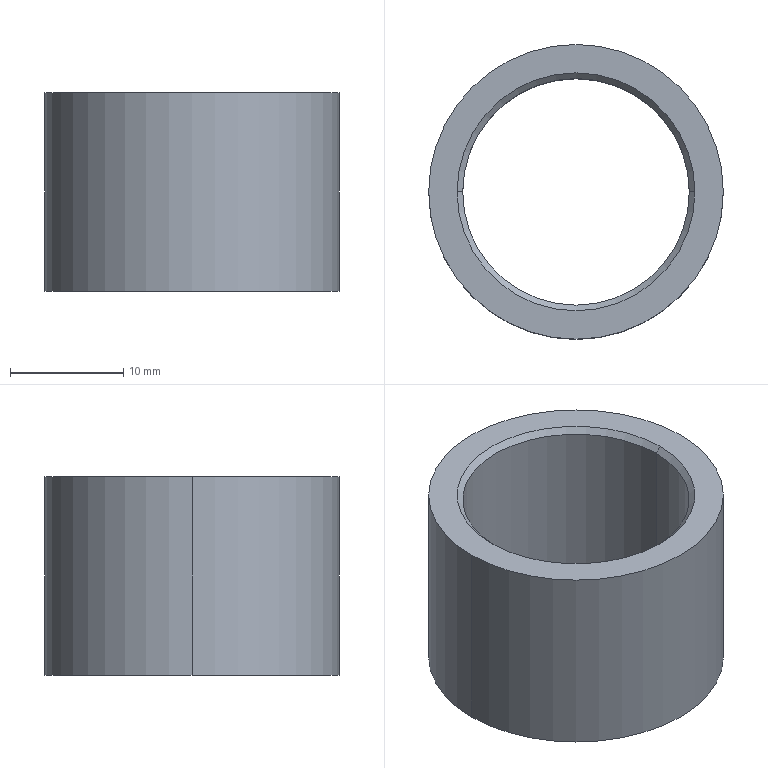Part | SolidWorks | features Chamfer 1, Extrusion 1 | 1 solid | 10 faces | box 26 x 26 x 17.5 mm | volume 3778 mm3 | cone 4 | cylinder 4 | plane 2 | commonest cylinder face diameters 20 x2 26 x2
STEP:
#1=CARTESIAN_POINT('',(-10.,0.,17.));
#2=VERTEX_POINT('',#1);
#3=CARTESIAN_POINT('',(10.,0.,17.));
#4=VERTEX_POINT('',#3);
#5=CARTESIAN_POINT('',(0.,0.,17.));
#6=DIRECTION('',(0.,0.,1.));
#7=DIRECTION('',(1.,0.,0.));
#8=AXIS2_PLACEMENT_3D('',#5,#6,#7);
#9=CIRCLE('',#8,10.);
#10=EDGE_CURVE('',#2,#4,#9,.T.);
#11=ORIENTED_EDGE('',*,*,#10,.F.);
#12=CARTESIAN_POINT('',(-10.5,0.,17.5));
#13=VERTEX_POINT('',#12);
#14=CARTESIAN_POINT('',(-10.,0.,17.));
#15=DIRECTION('',(-0.7071,0.,0.7071));
#16=VECTOR('',#15,1000.);
#17=LINE('',#14,#16);
#18=EDGE_CURVE('',#2,#13,#17,.T.);
#19=ORIENTED_EDGE('',*,*,#18,.T.);
#20=CARTESIAN_POINT('',(10.5,0.,17.5));
#21=VERTEX_POINT('',#20);
#22=CARTESIAN_POINT('',(0.,0.,17.5));
#23=DIRECTION('',(0.,0.,-1.));
#24=DIRECTION('',(1.,0.,0.));
#25=AXIS2_PLACEMENT_3D('',#22,#23,#24);
#26=CIRCLE('',#25,10.5);
#27=EDGE_CURVE('',#21,#13,#26,.T.);
#28=ORIENTED_EDGE('',*,*,#27,.F.);
#29=CARTESIAN_POINT('',(10.,0.,17.));
#30=DIRECTION('',(0.7071,0.,0.7071));
#31=VECTOR('',#30,1000.);
#32=LINE('',#29,#31);
#33=EDGE_CURVE('',#4,#21,#32,.T.);
#34=ORIENTED_EDGE('',*,*,#33,.F.);
#35=EDGE_LOOP('',(#11,#19,#28,#34));
#36=FACE_OUTER_BOUND('',#35,.T.);
#37=CARTESIAN_POINT('',(0.,0.,17.));
#38=DIRECTION('',(0.,0.,1.));
#39=DIRECTION('',(1.,0.,0.));
#40=AXIS2_PLACEMENT_3D('',#37,#38,#39);
#41=CONICAL_SURFACE('',#40,10.,0.7854);
#42=ADVANCED_FACE('',(#36),#41,.F.);
#43=CARTESIAN_POINT('',(10.,0.,0.5));
#44=VERTEX_POINT('',#43);
#45=CARTESIAN_POINT('',(-10.,0.,0.5));
#46=VERTEX_POINT('',#45);
#47=CARTESIAN_POINT('',(0.,0.,0.5));
#48=DIRECTION('',(0.,0.,-1.));
#49=DIRECTION('',(1.,0.,0.));
#50=AXIS2_PLACEMENT_3D('',#47,#48,#49);
#51=CIRCLE('',#50,10.);
#52=EDGE_CURVE('',#44,#46,#51,.T.);
#53=ORIENTED_EDGE('',*,*,#52,.F.);
#54=CARTESIAN_POINT('',(10.5,0.,0.));
#55=VERTEX_POINT('',#54);
#56=CARTESIAN_POINT('',(10.5,0.,0.));
#57=DIRECTION('',(0.7071,0.,-0.7071));
#58=VECTOR('',#57,1000.);
#59=LINE('',#56,#58);
#60=EDGE_CURVE('',#44,#55,#59,.T.);
#61=ORIENTED_EDGE('',*,*,#60,.T.);
#62=CARTESIAN_POINT('',(-10.5,0.,0.));
#63=VERTEX_POINT('',#62);
#64=CARTESIAN_POINT('',(0.,0.,0.));
#65=DIRECTION('',(0.,0.,1.));
#66=DIRECTION('',(1.,0.,0.));
#67=AXIS2_PLACEMENT_3D('',#64,#65,#66);
#68=CIRCLE('',#67,10.5);
#69=EDGE_CURVE('',#63,#55,#68,.T.);
#70=ORIENTED_EDGE('',*,*,#69,.F.);
#71=CARTESIAN_POINT('',(-10.5,0.,0.));
#72=DIRECTION('',(-0.7071,0.,-0.7071));
#73=VECTOR('',#72,1000.);
#74=LINE('',#71,#73);
#75=EDGE_CURVE('',#46,#63,#74,.T.);
#76=ORIENTED_EDGE('',*,*,#75,.F.);
#77=EDGE_LOOP('',(#53,#61,#70,#76));
#78=FACE_OUTER_BOUND('',#77,.T.);
#79=CARTESIAN_POINT('',(0.,0.,0.));
#80=DIRECTION('',(0.,0.,-1.));
#81=DIRECTION('',(-1.,0.,0.));
#82=AXIS2_PLACEMENT_3D('',#79,#80,#81);
#83=CONICAL_SURFACE('',#82,10.5,0.7854);
#84=ADVANCED_FACE('',(#78),#83,.F.);
#85=ORIENTED_EDGE('',*,*,#10,.T.);
#86=CARTESIAN_POINT('',(10.,0.,17.5));
#87=DIRECTION('',(0.,0.,-1.));
#88=VECTOR('',#87,1000.);
#89=LINE('',#86,#88);
#90=EDGE_CURVE('',#4,#44,#89,.T.);
#91=ORIENTED_EDGE('',*,*,#90,.T.);
#92=ORIENTED_EDGE('',*,*,#52,.T.);
#93=CARTESIAN_POINT('',(-10.,0.,17.5));
#94=DIRECTION('',(0.,0.,-1.));
#95=VECTOR('',#94,1000.);
#96=LINE('',#93,#95);
#97=EDGE_CURVE('',#2,#46,#96,.T.);
#98=ORIENTED_EDGE('',*,*,#97,.F.);
#99=EDGE_LOOP('',(#85,#91,#92,#98));
#100=FACE_OUTER_BOUND('',#99,.T.);
#101=CARTESIAN_POINT('',(0.,0.,17.5));
#102=DIRECTION('',(0.,0.,-1.));
#103=DIRECTION('',(-1.,0.,0.));
#104=AXIS2_PLACEMENT_3D('',#101,#102,#103);
#105=CYLINDRICAL_SURFACE('',#104,10.);
#106=ADVANCED_FACE('',(#100),#105,.F.);
#107=CARTESIAN_POINT('',(13.,0.,17.5));
#108=VERTEX_POINT('',#107);
#109=CARTESIAN_POINT('',(-13.,0.,17.5));
#110=VERTEX_POINT('',#109);
#111=CARTESIAN_POINT('',(0.,0.,17.5));
#112=DIRECTION('',(0.,0.,1.));
#113=DIRECTION('',(1.,0.,0.));
#114=AXIS2_PLACEMENT_3D('',#111,#112,#113);
#115=CIRCLE('',#114,13.);
#116=EDGE_CURVE('',#108,#110,#115,.T.);
#117=ORIENTED_EDGE('',*,*,#116,.F.);
#118=CARTESIAN_POINT('',(13.,0.,0.));
#119=VERTEX_POINT('',#118);
#120=CARTESIAN_POINT('',(13.,0.,17.5));
#121=DIRECTION('',(0.,0.,-1.));
#122=VECTOR('',#121,1000.);
#123=LINE('',#120,#122);
#124=EDGE_CURVE('',#108,#119,#123,.T.);
#125=ORIENTED_EDGE('',*,*,#124,.T.);
#126=CARTESIAN_POINT('',(-13.,0.,0.));
#127=VERTEX_POINT('',#126);
#128=CARTESIAN_POINT('',(0.,0.,0.));
#129=DIRECTION('',(0.,0.,1.));
#130=DIRECTION('',(1.,0.,0.));
#131=AXIS2_PLACEMENT_3D('',#128,#129,#130);
#132=CIRCLE('',#131,13.);
#133=EDGE_CURVE('',#119,#127,#132,.T.);
#134=ORIENTED_EDGE('',*,*,#133,.T.);
#135=CARTESIAN_POINT('',(-13.,0.,17.5));
#136=DIRECTION('',(0.,0.,-1.));
#137=VECTOR('',#136,1000.);
#138=LINE('',#135,#137);
#139=EDGE_CURVE('',#110,#127,#138,.T.);
#140=ORIENTED_EDGE('',*,*,#139,.F.);
#141=EDGE_LOOP('',(#117,#125,#134,#140));
#142=FACE_OUTER_BOUND('',#141,.T.);
#143=CARTESIAN_POINT('',(0.,0.,17.5));
#144=DIRECTION('',(0.,0.,-1.));
#145=DIRECTION('',(-1.,0.,0.));
#146=AXIS2_PLACEMENT_3D('',#143,#144,#145);
#147=CYLINDRICAL_SURFACE('',#146,13.);
#148=ADVANCED_FACE('',(#142),#147,.T.);
#149=ORIENTED_EDGE('',*,*,#27,.T.);
#150=CARTESIAN_POINT('',(0.,0.,17.5));
#151=DIRECTION('',(0.,0.,-1.));
#152=DIRECTION('',(1.,0.,0.));
#153=AXIS2_PLACEMENT_3D('',#150,#151,#152);
#154=CIRCLE('',#153,10.5);
#155=EDGE_CURVE('',#13,#21,#154,.T.);
#156=ORIENTED_EDGE('',*,*,#155,.T.);
#157=EDGE_LOOP('',(#149,#156));
#158=FACE_BOUND('',#157,.T.);
#159=CARTESIAN_POINT('',(0.,0.,17.5));
#160=DIRECTION('',(0.,0.,1.));
#161=DIRECTION('',(1.,0.,0.));
#162=AXIS2_PLACEMENT_3D('',#159,#160,#161);
#163=CIRCLE('',#162,13.);
#164=EDGE_CURVE('',#110,#108,#163,.T.);
#165=ORIENTED_EDGE('',*,*,#164,.T.);
#166=ORIENTED_EDGE('',*,*,#116,.T.);
#167=EDGE_LOOP('',(#165,#166));
#168=FACE_OUTER_BOUND('',#167,.T.);
#169=CARTESIAN_POINT('',(0.,0.,17.5));
#170=DIRECTION('',(0.,0.,1.));
#171=DIRECTION('',(1.,0.,0.));
#172=AXIS2_PLACEMENT_3D('',#169,#170,#171);
#173=PLANE('',#172);
#174=ADVANCED_FACE('',(#158,#168),#173,.T.);
#175=ORIENTED_EDGE('',*,*,#69,.T.);
#176=CARTESIAN_POINT('',(0.,0.,0.));
#177=DIRECTION('',(0.,0.,1.));
#178=DIRECTION('',(1.,0.,0.));
#179=AXIS2_PLACEMENT_3D('',#176,#177,#178);
#180=CIRCLE('',#179,10.5);
#181=EDGE_CURVE('',#55,#63,#180,.T.);
#182=ORIENTED_EDGE('',*,*,#181,.T.);
#183=EDGE_LOOP('',(#175,#182));
#184=FACE_BOUND('',#183,.T.);
#185=CARTESIAN_POINT('',(0.,0.,0.));
#186=DIRECTION('',(0.,0.,1.));
#187=DIRECTION('',(1.,0.,0.));
#188=AXIS2_PLACEMENT_3D('',#185,#186,#187);
#189=CIRCLE('',#188,13.);
#190=EDGE_CURVE('',#127,#119,#189,.T.);
#191=ORIENTED_EDGE('',*,*,#190,.F.);
#192=ORIENTED_EDGE('',*,*,#133,.F.);
#193=EDGE_LOOP('',(#191,#192));
#194=FACE_OUTER_BOUND('',#193,.T.);
#195=CARTESIAN_POINT('',(0.,0.,0.));
#196=DIRECTION('',(0.,0.,1.));
#197=DIRECTION('',(1.,0.,0.));
#198=AXIS2_PLACEMENT_3D('',#195,#196,#197);
#199=PLANE('',#198);
#200=ADVANCED_FACE('',(#184,#194),#199,.F.);
#201=ORIENTED_EDGE('',*,*,#124,.F.);
#202=ORIENTED_EDGE('',*,*,#164,.F.);
#203=ORIENTED_EDGE('',*,*,#139,.T.);
#204=ORIENTED_EDGE('',*,*,#190,.T.);
#205=EDGE_LOOP('',(#201,#202,#203,#204));
#206=FACE_OUTER_BOUND('',#205,.T.);
#207=CARTESIAN_POINT('',(0.,0.,17.5));
#208=DIRECTION('',(0.,0.,-1.));
#209=DIRECTION('',(-1.,0.,0.));
#210=AXIS2_PLACEMENT_3D('',#207,#208,#209);
#211=CYLINDRICAL_SURFACE('',#210,13.);
#212=ADVANCED_FACE('',(#206),#211,.T.);
#213=ORIENTED_EDGE('',*,*,#90,.F.);
#214=CARTESIAN_POINT('',(0.,0.,17.));
#215=DIRECTION('',(0.,0.,1.));
#216=DIRECTION('',(1.,0.,0.));
#217=AXIS2_PLACEMENT_3D('',#214,#215,#216);
#218=CIRCLE('',#217,10.);
#219=EDGE_CURVE('',#4,#2,#218,.T.);
#220=ORIENTED_EDGE('',*,*,#219,.T.);
#221=ORIENTED_EDGE('',*,*,#97,.T.);
#222=CARTESIAN_POINT('',(0.,0.,0.5));
#223=DIRECTION('',(0.,0.,-1.));
#224=DIRECTION('',(1.,0.,0.));
#225=AXIS2_PLACEMENT_3D('',#222,#223,#224);
#226=CIRCLE('',#225,10.);
#227=EDGE_CURVE('',#46,#44,#226,.T.);
#228=ORIENTED_EDGE('',*,*,#227,.T.);
#229=EDGE_LOOP('',(#213,#220,#221,#228));
#230=FACE_OUTER_BOUND('',#229,.T.);
#231=CARTESIAN_POINT('',(0.,0.,17.5));
#232=DIRECTION('',(0.,0.,-1.));
#233=DIRECTION('',(-1.,0.,0.));
#234=AXIS2_PLACEMENT_3D('',#231,#232,#233);
#235=CYLINDRICAL_SURFACE('',#234,10.);
#236=ADVANCED_FACE('',(#230),#235,.F.);
#237=ORIENTED_EDGE('',*,*,#60,.F.);
#238=ORIENTED_EDGE('',*,*,#227,.F.);
#239=ORIENTED_EDGE('',*,*,#75,.T.);
#240=ORIENTED_EDGE('',*,*,#181,.F.);
#241=EDGE_LOOP('',(#237,#238,#239,#240));
#242=FACE_OUTER_BOUND('',#241,.T.);
#243=CARTESIAN_POINT('',(0.,0.,0.));
#244=DIRECTION('',(0.,0.,-1.));
#245=DIRECTION('',(-1.,0.,0.));
#246=AXIS2_PLACEMENT_3D('',#243,#244,#245);
#247=CONICAL_SURFACE('',#246,10.5,0.7854);
#248=ADVANCED_FACE('',(#242),#247,.F.);
#249=ORIENTED_EDGE('',*,*,#18,.F.);
#250=ORIENTED_EDGE('',*,*,#219,.F.);
#251=ORIENTED_EDGE('',*,*,#33,.T.);
#252=ORIENTED_EDGE('',*,*,#155,.F.);
#253=EDGE_LOOP('',(#249,#250,#251,#252));
#254=FACE_OUTER_BOUND('',#253,.T.);
#255=CARTESIAN_POINT('',(0.,0.,17.));
#256=DIRECTION('',(0.,0.,1.));
#257=DIRECTION('',(1.,0.,0.));
#258=AXIS2_PLACEMENT_3D('',#255,#256,#257);
#259=CONICAL_SURFACE('',#258,10.,0.7854);
#260=ADVANCED_FACE('',(#254),#259,.F.);
#261=CLOSED_SHELL('',(#42,#84,#106,#148,#174,#200,#212,#236,#248,#260));
#262=MANIFOLD_SOLID_BREP('',#261);
#263=CARTESIAN_POINT('',(0.,0.,0.));
#264=DIRECTION('',(0.,0.,1.));
#265=DIRECTION('',(1.,0.,0.));
#266=AXIS2_PLACEMENT_3D('',#263,#264,#265);
#267=(LENGTH_UNIT()NAMED_UNIT(*)SI_UNIT(.MILLI.,.METRE.));
#268=UNCERTAINTY_MEASURE_WITH_UNIT(LENGTH_MEASURE(0.00001),#267,'','');
#269=(NAMED_UNIT(*)PLANE_ANGLE_UNIT()SI_UNIT($,.RADIAN.));
#270=(NAMED_UNIT(*)SI_UNIT($,.STERADIAN.)SOLID_ANGLE_UNIT());
#271=(GEOMETRIC_REPRESENTATION_CONTEXT(3)GLOBAL_UNCERTAINTY_ASSIGNED_CONTEXT((#268))GLOBAL_UNIT_ASSIGNED_CONTEXT((#267,#269,#270))REPRESENTATION_CONTEXT('',''));
#272=ADVANCED_BREP_SHAPE_REPRESENTATION('',(#262,#266),#271);